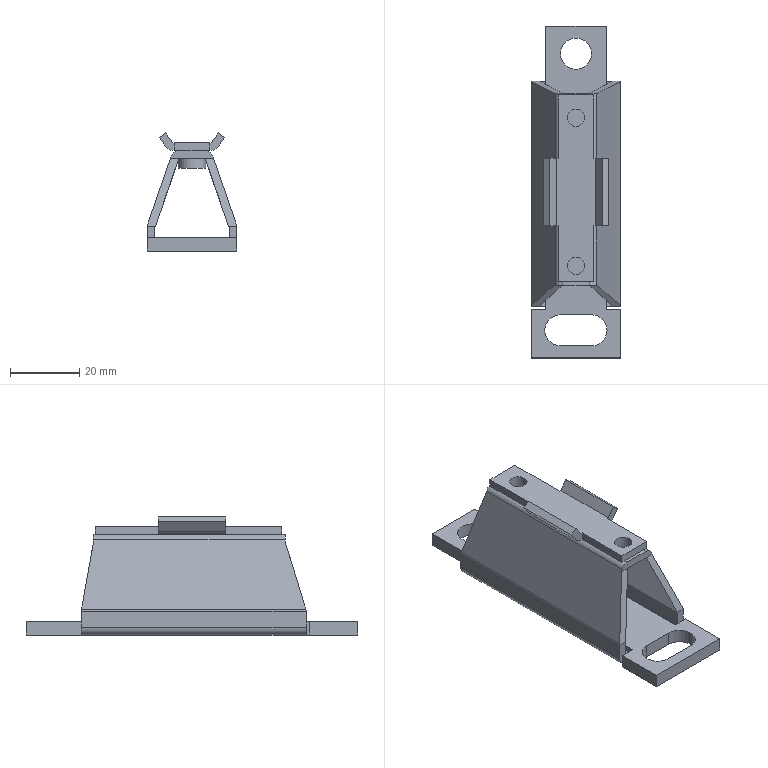Part | STEP file | AC40-04-KSTV-38JNR_AC3009A Spacer Rear Plate(4T) | 1 solid | 78 faces | box 26 x 96 x 34.173 mm | volume 17760 mm3 | plane 56 | cylinder 22 | commonest cylinder face diameters 4.6 x8 8 x5 9 x5 5 x4